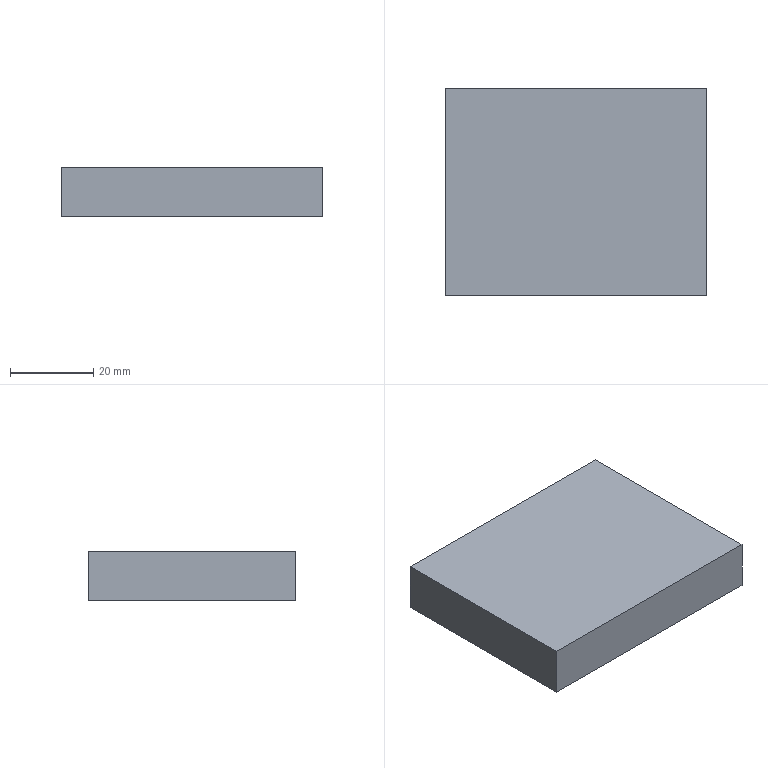Part | SolidWorks | features FlatPattern 1, SMBaseFlange 1, SheetMetal 1 | 1 solid | 6 faces | box 63 x 50 x 12 mm | volume 37800 mm3 | plane 6
STEP:
#1=CARTESIAN_POINT('',(40.222,-296.937,0.));
#2=VERTEX_POINT('',#1);
#3=CARTESIAN_POINT('',(40.222,-246.937,0.));
#4=VERTEX_POINT('',#3);
#5=CARTESIAN_POINT('',(40.222,-296.937,0.));
#6=DIRECTION('',(0.,1.,0.));
#7=VECTOR('',#6,1000.);
#8=LINE('',#5,#7);
#9=EDGE_CURVE('',#2,#4,#8,.T.);
#10=ORIENTED_EDGE('',*,*,#9,.F.);
#11=CARTESIAN_POINT('',(40.222,-296.937,-12.));
#12=VERTEX_POINT('',#11);
#13=CARTESIAN_POINT('',(40.222,-296.937,-12.));
#14=DIRECTION('',(0.,0.,1.));
#15=VECTOR('',#14,1000.);
#16=LINE('',#13,#15);
#17=EDGE_CURVE('',#12,#2,#16,.T.);
#18=ORIENTED_EDGE('',*,*,#17,.F.);
#19=CARTESIAN_POINT('',(40.222,-246.937,-12.));
#20=VERTEX_POINT('',#19);
#21=CARTESIAN_POINT('',(40.222,-296.937,-12.));
#22=DIRECTION('',(0.,1.,0.));
#23=VECTOR('',#22,1000.);
#24=LINE('',#21,#23);
#25=EDGE_CURVE('',#12,#20,#24,.T.);
#26=ORIENTED_EDGE('',*,*,#25,.T.);
#27=CARTESIAN_POINT('',(40.222,-246.937,-12.));
#28=DIRECTION('',(0.,0.,1.));
#29=VECTOR('',#28,1000.);
#30=LINE('',#27,#29);
#31=EDGE_CURVE('',#20,#4,#30,.T.);
#32=ORIENTED_EDGE('',*,*,#31,.T.);
#33=EDGE_LOOP('',(#10,#18,#26,#32));
#34=FACE_OUTER_BOUND('',#33,.T.);
#35=CARTESIAN_POINT('',(40.222,-296.937,-12.));
#36=DIRECTION('',(1.,0.,0.));
#37=DIRECTION('',(0.,0.,-1.));
#38=AXIS2_PLACEMENT_3D('',#35,#36,#37);
#39=PLANE('',#38);
#40=ADVANCED_FACE('',(#34),#39,.T.);
#41=CARTESIAN_POINT('',(-22.778,-296.937,0.));
#42=VERTEX_POINT('',#41);
#43=CARTESIAN_POINT('',(40.222,-296.937,0.));
#44=DIRECTION('',(1.,0.,0.));
#45=VECTOR('',#44,1000.);
#46=LINE('',#43,#45);
#47=EDGE_CURVE('',#42,#2,#46,.T.);
#48=ORIENTED_EDGE('',*,*,#47,.F.);
#49=CARTESIAN_POINT('',(-22.778,-296.937,-12.));
#50=VERTEX_POINT('',#49);
#51=CARTESIAN_POINT('',(-22.778,-296.937,-12.));
#52=DIRECTION('',(0.,0.,1.));
#53=VECTOR('',#52,1000.);
#54=LINE('',#51,#53);
#55=EDGE_CURVE('',#50,#42,#54,.T.);
#56=ORIENTED_EDGE('',*,*,#55,.F.);
#57=CARTESIAN_POINT('',(40.222,-296.937,-12.));
#58=DIRECTION('',(1.,0.,0.));
#59=VECTOR('',#58,1000.);
#60=LINE('',#57,#59);
#61=EDGE_CURVE('',#50,#12,#60,.T.);
#62=ORIENTED_EDGE('',*,*,#61,.T.);
#63=ORIENTED_EDGE('',*,*,#17,.T.);
#64=EDGE_LOOP('',(#48,#56,#62,#63));
#65=FACE_OUTER_BOUND('',#64,.T.);
#66=CARTESIAN_POINT('',(40.222,-296.937,-12.));
#67=DIRECTION('',(0.,-1.,0.));
#68=DIRECTION('',(0.,0.,-1.));
#69=AXIS2_PLACEMENT_3D('',#66,#67,#68);
#70=PLANE('',#69);
#71=ADVANCED_FACE('',(#65),#70,.T.);
#72=CARTESIAN_POINT('',(-22.778,-246.937,0.));
#73=VERTEX_POINT('',#72);
#74=CARTESIAN_POINT('',(-22.778,-296.937,0.));
#75=DIRECTION('',(0.,-1.,0.));
#76=VECTOR('',#75,1000.);
#77=LINE('',#74,#76);
#78=EDGE_CURVE('',#73,#42,#77,.T.);
#79=ORIENTED_EDGE('',*,*,#78,.F.);
#80=CARTESIAN_POINT('',(-22.778,-246.937,-12.));
#81=VERTEX_POINT('',#80);
#82=CARTESIAN_POINT('',(-22.778,-246.937,-12.));
#83=DIRECTION('',(0.,0.,1.));
#84=VECTOR('',#83,1000.);
#85=LINE('',#82,#84);
#86=EDGE_CURVE('',#81,#73,#85,.T.);
#87=ORIENTED_EDGE('',*,*,#86,.F.);
#88=CARTESIAN_POINT('',(-22.778,-296.937,-12.));
#89=DIRECTION('',(0.,-1.,0.));
#90=VECTOR('',#89,1000.);
#91=LINE('',#88,#90);
#92=EDGE_CURVE('',#81,#50,#91,.T.);
#93=ORIENTED_EDGE('',*,*,#92,.T.);
#94=ORIENTED_EDGE('',*,*,#55,.T.);
#95=EDGE_LOOP('',(#79,#87,#93,#94));
#96=FACE_OUTER_BOUND('',#95,.T.);
#97=CARTESIAN_POINT('',(-22.778,-296.937,-12.));
#98=DIRECTION('',(-1.,0.,0.));
#99=DIRECTION('',(0.,0.,1.));
#100=AXIS2_PLACEMENT_3D('',#97,#98,#99);
#101=PLANE('',#100);
#102=ADVANCED_FACE('',(#96),#101,.T.);
#103=CARTESIAN_POINT('',(40.222,-246.937,0.));
#104=DIRECTION('',(-1.,0.,0.));
#105=VECTOR('',#104,1000.);
#106=LINE('',#103,#105);
#107=EDGE_CURVE('',#4,#73,#106,.T.);
#108=ORIENTED_EDGE('',*,*,#107,.F.);
#109=ORIENTED_EDGE('',*,*,#31,.F.);
#110=CARTESIAN_POINT('',(40.222,-246.937,-12.));
#111=DIRECTION('',(-1.,0.,0.));
#112=VECTOR('',#111,1000.);
#113=LINE('',#110,#112);
#114=EDGE_CURVE('',#20,#81,#113,.T.);
#115=ORIENTED_EDGE('',*,*,#114,.T.);
#116=ORIENTED_EDGE('',*,*,#86,.T.);
#117=EDGE_LOOP('',(#108,#109,#115,#116));
#118=FACE_OUTER_BOUND('',#117,.T.);
#119=CARTESIAN_POINT('',(40.222,-246.937,-12.));
#120=DIRECTION('',(0.,1.,0.));
#121=DIRECTION('',(0.,0.,1.));
#122=AXIS2_PLACEMENT_3D('',#119,#120,#121);
#123=PLANE('',#122);
#124=ADVANCED_FACE('',(#118),#123,.T.);
#125=ORIENTED_EDGE('',*,*,#25,.F.);
#126=ORIENTED_EDGE('',*,*,#61,.F.);
#127=ORIENTED_EDGE('',*,*,#92,.F.);
#128=ORIENTED_EDGE('',*,*,#114,.F.);
#129=EDGE_LOOP('',(#125,#126,#127,#128));
#130=FACE_OUTER_BOUND('',#129,.T.);
#131=CARTESIAN_POINT('',(0.,0.,-12.));
#132=DIRECTION('',(0.,0.,1.));
#133=DIRECTION('',(1.,0.,0.));
#134=AXIS2_PLACEMENT_3D('',#131,#132,#133);
#135=PLANE('',#134);
#136=ADVANCED_FACE('',(#130),#135,.F.);
#137=ORIENTED_EDGE('',*,*,#9,.T.);
#138=ORIENTED_EDGE('',*,*,#107,.T.);
#139=ORIENTED_EDGE('',*,*,#78,.T.);
#140=ORIENTED_EDGE('',*,*,#47,.T.);
#141=EDGE_LOOP('',(#137,#138,#139,#140));
#142=FACE_OUTER_BOUND('',#141,.T.);
#143=CARTESIAN_POINT('',(0.,0.,0.));
#144=DIRECTION('',(0.,0.,1.));
#145=DIRECTION('',(1.,0.,0.));
#146=AXIS2_PLACEMENT_3D('',#143,#144,#145);
#147=PLANE('',#146);
#148=ADVANCED_FACE('',(#142),#147,.T.);
#149=CLOSED_SHELL('',(#40,#71,#102,#124,#136,#148));
#150=MANIFOLD_SOLID_BREP('',#149);
#151=CARTESIAN_POINT('',(0.,0.,0.));
#152=DIRECTION('',(0.,0.,1.));
#153=DIRECTION('',(1.,0.,0.));
#154=AXIS2_PLACEMENT_3D('',#151,#152,#153);
#155=(LENGTH_UNIT()NAMED_UNIT(*)SI_UNIT(.MILLI.,.METRE.));
#156=UNCERTAINTY_MEASURE_WITH_UNIT(LENGTH_MEASURE(0.00001),#155,'','');
#157=(NAMED_UNIT(*)PLANE_ANGLE_UNIT()SI_UNIT($,.RADIAN.));
#158=(NAMED_UNIT(*)SI_UNIT($,.STERADIAN.)SOLID_ANGLE_UNIT());
#159=(GEOMETRIC_REPRESENTATION_CONTEXT(3)GLOBAL_UNCERTAINTY_ASSIGNED_CONTEXT((#156))GLOBAL_UNIT_ASSIGNED_CONTEXT((#155,#157,#158))REPRESENTATION_CONTEXT('',''));
#160=ADVANCED_BREP_SHAPE_REPRESENTATION('',(#150,#154),#159);